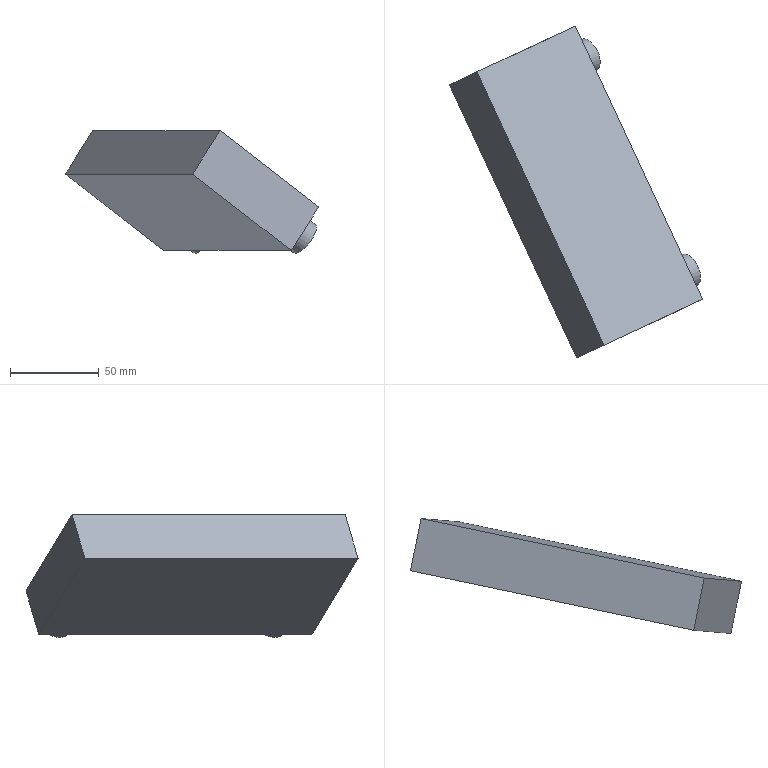Part | NX | features solid 2 | 1 solid | 10 faces | box 143.12 x 187.309 x 69.233 mm | volume 388783 mm3 | plane 8 | cylinder 2 | commonest cylinder face diameters 20 x2
STEP:
#1=CARTESIAN_POINT('',(1191.659,789.264,-190.085));
#2=VERTEX_POINT('',#1);
#3=CARTESIAN_POINT('',(1119.814,943.336,-190.085));
#4=VERTEX_POINT('',#3);
#5=CARTESIAN_POINT('',(1050.082,1092.877,-190.085));
#6=DIRECTION('',(-0.4226,0.9063,0.000000003));
#7=VECTOR('',#6,1000.);
#8=LINE('',#5,#7);
#9=EDGE_CURVE('',#2,#4,#8,.T.);
#10=ORIENTED_EDGE('',*,*,#9,.T.);
#11=CARTESIAN_POINT('',(1064.134,917.372,-147.066));
#12=VERTEX_POINT('',#11);
#13=CARTESIAN_POINT('',(1064.134,917.372,-147.066));
#14=DIRECTION('',(0.7424,0.3462,-0.5736));
#15=VECTOR('',#14,1000.);
#16=LINE('',#13,#15);
#17=EDGE_CURVE('',#12,#4,#16,.T.);
#18=ORIENTED_EDGE('',*,*,#17,.F.);
#19=CARTESIAN_POINT('',(1135.979,763.3,-147.066));
#20=VERTEX_POINT('',#19);
#21=CARTESIAN_POINT('',(994.402,1066.913,-147.066));
#22=DIRECTION('',(-0.4226,0.9063,0.000000003));
#23=VECTOR('',#22,1000.);
#24=LINE('',#21,#23);
#25=EDGE_CURVE('',#20,#12,#24,.T.);
#26=ORIENTED_EDGE('',*,*,#25,.F.);
#27=CARTESIAN_POINT('',(1135.979,763.3,-147.066));
#28=DIRECTION('',(-0.7424,-0.3462,0.5736));
#29=VECTOR('',#28,1000.);
#30=LINE('',#27,#29);
#31=EDGE_CURVE('',#2,#20,#30,.T.);
#32=ORIENTED_EDGE('',*,*,#31,.F.);
#33=EDGE_LOOP('',(#10,#18,#26,#32));
#34=FACE_BOUND('',#33,.T.);
#35=CARTESIAN_POINT('',(1142.318,749.705,-147.066));
#36=DIRECTION('',(0.5198,0.2424,0.8192));
#37=DIRECTION('',(0.7424,0.3462,-0.5736));
#38=AXIS2_PLACEMENT_3D('',#35,#36,#37);
#39=PLANE('',#38);
#40=ADVANCED_FACE('',(#34),#39,.T.);
#41=CARTESIAN_POINT('',(1176.064,781.992,-214.659));
#42=VERTEX_POINT('',#41);
#43=CARTESIAN_POINT('',(1104.219,936.064,-214.659));
#44=VERTEX_POINT('',#43);
#45=CARTESIAN_POINT('',(1034.487,1085.605,-214.659));
#46=DIRECTION('',(-0.4226,0.9063,0.000000003));
#47=VECTOR('',#46,1000.);
#48=LINE('',#45,#47);
#49=EDGE_CURVE('',#42,#44,#48,.T.);
#50=ORIENTED_EDGE('',*,*,#49,.F.);
#51=CARTESIAN_POINT('',(1120.384,756.028,-171.641));
#52=VERTEX_POINT('',#51);
#53=CARTESIAN_POINT('',(1120.384,756.028,-171.641));
#54=DIRECTION('',(-0.7424,-0.3462,0.5736));
#55=VECTOR('',#54,1000.);
#56=LINE('',#53,#55);
#57=EDGE_CURVE('',#42,#52,#56,.T.);
#58=ORIENTED_EDGE('',*,*,#57,.T.);
#59=CARTESIAN_POINT('',(1048.539,910.1,-171.641));
#60=VERTEX_POINT('',#59);
#61=CARTESIAN_POINT('',(978.807,1059.641,-171.641));
#62=DIRECTION('',(-0.4226,0.9063,0.000000003));
#63=VECTOR('',#62,1000.);
#64=LINE('',#61,#63);
#65=EDGE_CURVE('',#52,#60,#64,.T.);
#66=ORIENTED_EDGE('',*,*,#65,.T.);
#67=CARTESIAN_POINT('',(1048.539,910.1,-171.641));
#68=DIRECTION('',(0.7424,0.3462,-0.5736));
#69=VECTOR('',#68,1000.);
#70=LINE('',#67,#69);
#71=EDGE_CURVE('',#60,#44,#70,.T.);
#72=ORIENTED_EDGE('',*,*,#71,.T.);
#73=EDGE_LOOP('',(#50,#58,#66,#72));
#74=FACE_BOUND('',#73,.T.);
#75=CARTESIAN_POINT('',(1126.723,742.433,-171.641));
#76=DIRECTION('',(0.5198,0.2424,0.8192));
#77=DIRECTION('',(0.7424,0.3462,-0.5736));
#78=AXIS2_PLACEMENT_3D('',#75,#76,#77);
#79=PLANE('',#78);
#80=ADVANCED_FACE('',(#74),#79,.F.);
#81=ORIENTED_EDGE('',*,*,#17,.T.);
#82=CARTESIAN_POINT('',(1136.969,951.336,-163.053));
#83=DIRECTION('',(-0.5198,-0.2424,-0.8192));
#84=VECTOR('',#83,1000.);
#85=LINE('',#82,#84);
#86=EDGE_CURVE('',#4,#44,#85,.T.);
#87=ORIENTED_EDGE('',*,*,#86,.T.);
#88=ORIENTED_EDGE('',*,*,#71,.F.);
#89=CARTESIAN_POINT('',(1081.288,925.371,-120.034));
#90=DIRECTION('',(-0.5198,-0.2424,-0.8192));
#91=VECTOR('',#90,1000.);
#92=LINE('',#89,#91);
#93=EDGE_CURVE('',#12,#60,#92,.T.);
#94=ORIENTED_EDGE('',*,*,#93,.F.);
#95=EDGE_LOOP('',(#81,#87,#88,#94));
#96=FACE_BOUND('',#95,.T.);
#97=CARTESIAN_POINT('',(1081.288,925.371,-120.034));
#98=DIRECTION('',(0.4226,-0.9063,-0.000000003));
#99=DIRECTION('',(0.8754,0.4082,-0.2588));
#100=AXIS2_PLACEMENT_3D('',#97,#98,#99);
#101=PLANE('',#100);
#102=ADVANCED_FACE('',(#96),#101,.F.);
#103=ORIENTED_EDGE('',*,*,#31,.T.);
#104=CARTESIAN_POINT('',(1153.133,771.299,-120.034));
#105=DIRECTION('',(-0.5198,-0.2424,-0.8192));
#106=VECTOR('',#105,1000.);
#107=LINE('',#104,#106);
#108=EDGE_CURVE('',#20,#52,#107,.T.);
#109=ORIENTED_EDGE('',*,*,#108,.T.);
#110=ORIENTED_EDGE('',*,*,#57,.F.);
#111=CARTESIAN_POINT('',(1208.814,797.263,-163.053));
#112=DIRECTION('',(-0.5198,-0.2424,-0.8192));
#113=VECTOR('',#112,1000.);
#114=LINE('',#111,#113);
#115=EDGE_CURVE('',#2,#42,#114,.T.);
#116=ORIENTED_EDGE('',*,*,#115,.F.);
#117=EDGE_LOOP('',(#103,#109,#110,#116));
#118=FACE_BOUND('',#117,.T.);
#119=CARTESIAN_POINT('',(1153.133,771.299,-120.034));
#120=DIRECTION('',(-0.4226,0.9063,0.000000003));
#121=DIRECTION('',(0.8754,0.4082,-0.2588));
#122=AXIS2_PLACEMENT_3D('',#119,#120,#121);
#123=PLANE('',#122);
#124=ADVANCED_FACE('',(#118),#123,.F.);
#125=CARTESIAN_POINT('',(1114.425,920.963,-210.563));
#126=VERTEX_POINT('',#125);
#127=CARTESIAN_POINT('',(1119.624,923.387,-202.372));
#128=DIRECTION('',(-0.7424,-0.3462,0.5736));
#129=DIRECTION('',(-0.5198,-0.2424,-0.8192));
#130=AXIS2_PLACEMENT_3D('',#127,#128,#129);
#131=CIRCLE('',#130,10.);
#132=EDGE_CURVE('',#126,#126,#131,.T.);
#133=ORIENTED_EDGE('',*,*,#132,.T.);
#134=EDGE_LOOP('',(#133));
#135=FACE_BOUND('',#134,.T.);
#136=CARTESIAN_POINT('',(1171.056,799.517,-210.563));
#137=VERTEX_POINT('',#136);
#138=CARTESIAN_POINT('',(1176.254,801.941,-202.372));
#139=DIRECTION('',(-0.7424,-0.3462,0.5736));
#140=DIRECTION('',(-0.5198,-0.2424,-0.8192));
#141=AXIS2_PLACEMENT_3D('',#138,#139,#140);
#142=CIRCLE('',#141,10.);
#143=EDGE_CURVE('',#137,#137,#142,.T.);
#144=ORIENTED_EDGE('',*,*,#143,.T.);
#145=EDGE_LOOP('',(#144));
#146=FACE_BOUND('',#145,.T.);
#147=ORIENTED_EDGE('',*,*,#115,.T.);
#148=ORIENTED_EDGE('',*,*,#49,.T.);
#149=ORIENTED_EDGE('',*,*,#86,.F.);
#150=ORIENTED_EDGE('',*,*,#9,.F.);
#151=EDGE_LOOP('',(#147,#148,#149,#150));
#152=FACE_BOUND('',#151,.T.);
#153=CARTESIAN_POINT('',(1067.237,1100.876,-163.053));
#154=DIRECTION('',(0.7424,0.3462,-0.5736));
#155=DIRECTION('',(-0.5198,-0.2424,-0.8192));
#156=AXIS2_PLACEMENT_3D('',#153,#154,#155);
#157=PLANE('',#156);
#158=ADVANCED_FACE('',(#135,#146,#152),#157,.T.);
#159=ORIENTED_EDGE('',*,*,#25,.T.);
#160=ORIENTED_EDGE('',*,*,#93,.T.);
#161=ORIENTED_EDGE('',*,*,#65,.F.);
#162=ORIENTED_EDGE('',*,*,#108,.F.);
#163=EDGE_LOOP('',(#159,#160,#161,#162));
#164=FACE_BOUND('',#163,.T.);
#165=CARTESIAN_POINT('',(978.807,1059.641,-171.641));
#166=DIRECTION('',(0.7424,0.3462,-0.5736));
#167=DIRECTION('',(-0.5198,-0.2424,-0.8192));
#168=AXIS2_PLACEMENT_3D('',#165,#166,#167);
#169=PLANE('',#168);
#170=ADVANCED_FACE('',(#164),#169,.F.);
#171=CARTESIAN_POINT('',(1178.48,802.979,-216.299));
#172=VERTEX_POINT('',#171);
#173=CARTESIAN_POINT('',(1183.678,805.403,-208.108));
#174=DIRECTION('',(-0.7424,-0.3462,0.5736));
#175=DIRECTION('',(-0.5198,-0.2424,-0.8192));
#176=AXIS2_PLACEMENT_3D('',#173,#174,#175);
#177=CIRCLE('',#176,10.);
#178=EDGE_CURVE('',#172,#172,#177,.T.);
#179=ORIENTED_EDGE('',*,*,#178,.F.);
#180=EDGE_LOOP('',(#179));
#181=FACE_BOUND('',#180,.T.);
#182=CARTESIAN_POINT('',(1183.678,805.403,-208.108));
#183=DIRECTION('',(0.7424,0.3462,-0.5736));
#184=DIRECTION('',(-0.5198,-0.2424,-0.8192));
#185=AXIS2_PLACEMENT_3D('',#182,#183,#184);
#186=PLANE('',#185);
#187=ADVANCED_FACE('',(#181),#186,.T.);
#188=ORIENTED_EDGE('',*,*,#178,.T.);
#189=EDGE_LOOP('',(#188));
#190=FACE_BOUND('',#189,.T.);
#191=ORIENTED_EDGE('',*,*,#143,.F.);
#192=EDGE_LOOP('',(#191));
#193=FACE_BOUND('',#192,.T.);
#194=CARTESIAN_POINT('',(1168.83,798.48,-196.636));
#195=DIRECTION('',(0.7424,0.3462,-0.5736));
#196=DIRECTION('',(-0.5198,-0.2424,-0.8192));
#197=AXIS2_PLACEMENT_3D('',#194,#195,#196);
#198=CYLINDRICAL_SURFACE('',#197,10.);
#199=ADVANCED_FACE('',(#190,#193),#198,.T.);
#200=CARTESIAN_POINT('',(1121.849,924.425,-216.299));
#201=VERTEX_POINT('',#200);
#202=CARTESIAN_POINT('',(1127.048,926.849,-208.108));
#203=DIRECTION('',(-0.7424,-0.3462,0.5736));
#204=DIRECTION('',(-0.5198,-0.2424,-0.8192));
#205=AXIS2_PLACEMENT_3D('',#202,#203,#204);
#206=CIRCLE('',#205,10.);
#207=EDGE_CURVE('',#201,#201,#206,.T.);
#208=ORIENTED_EDGE('',*,*,#207,.F.);
#209=EDGE_LOOP('',(#208));
#210=FACE_BOUND('',#209,.T.);
#211=CARTESIAN_POINT('',(1127.048,926.849,-208.108));
#212=DIRECTION('',(0.7424,0.3462,-0.5736));
#213=DIRECTION('',(-0.5198,-0.2424,-0.8192));
#214=AXIS2_PLACEMENT_3D('',#211,#212,#213);
#215=PLANE('',#214);
#216=ADVANCED_FACE('',(#210),#215,.T.);
#217=ORIENTED_EDGE('',*,*,#207,.T.);
#218=EDGE_LOOP('',(#217));
#219=FACE_BOUND('',#218,.T.);
#220=ORIENTED_EDGE('',*,*,#132,.F.);
#221=EDGE_LOOP('',(#220));
#222=FACE_BOUND('',#221,.T.);
#223=CARTESIAN_POINT('',(1112.2,919.925,-196.636));
#224=DIRECTION('',(0.7424,0.3462,-0.5736));
#225=DIRECTION('',(-0.5198,-0.2424,-0.8192));
#226=AXIS2_PLACEMENT_3D('',#223,#224,#225);
#227=CYLINDRICAL_SURFACE('',#226,10.);
#228=ADVANCED_FACE('',(#219,#222),#227,.T.);
#229=CLOSED_SHELL('',(#40,#80,#102,#124,#158,#170,#187,#199,#216,#228));
#230=MANIFOLD_SOLID_BREP('',#229);
#231=(LENGTH_UNIT()NAMED_UNIT(*)SI_UNIT(.MILLI.,.METRE.));
#232=UNCERTAINTY_MEASURE_WITH_UNIT(LENGTH_MEASURE(0.00001),#231,'','');
#233=(NAMED_UNIT(*)PLANE_ANGLE_UNIT()SI_UNIT($,.RADIAN.));
#234=(NAMED_UNIT(*)SI_UNIT($,.STERADIAN.)SOLID_ANGLE_UNIT());
#235=(GEOMETRIC_REPRESENTATION_CONTEXT(3)GLOBAL_UNCERTAINTY_ASSIGNED_CONTEXT((#232))GLOBAL_UNIT_ASSIGNED_CONTEXT((#231,#233,#234))REPRESENTATION_CONTEXT('',''));
#236=ADVANCED_BREP_SHAPE_REPRESENTATION('',(#230),#235);